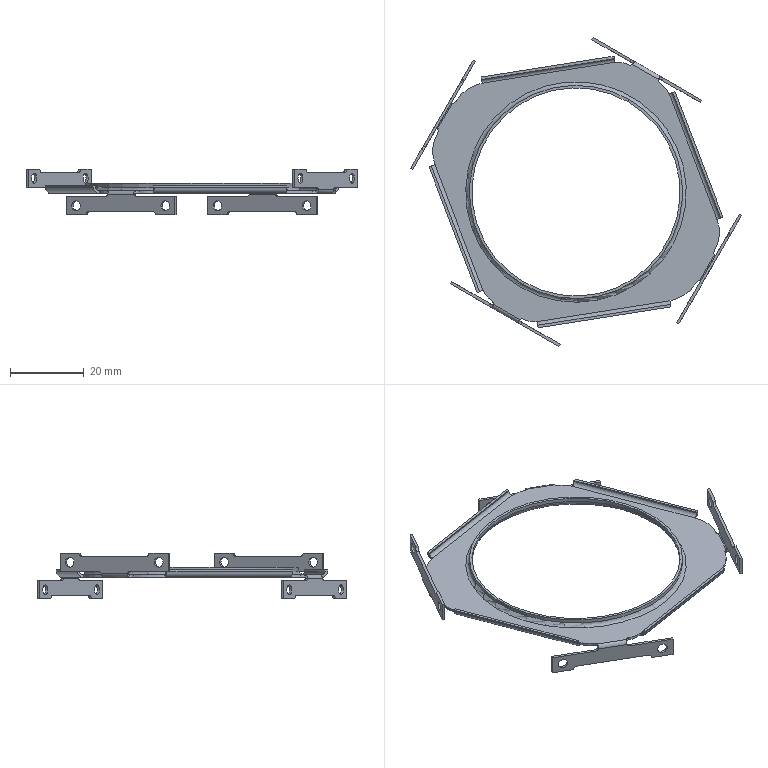Part | STEP file | 1 solid | 128 faces | box 90.075 x 84.017 x 12.5 mm | volume 2024 mm3 | plane 60 | cylinder 58 | spline 8 | torus 2 | commonest cylinder face diameters 2 x32 2.7 x8 0.6 x4 3.4 x4 12 x4 20 x4